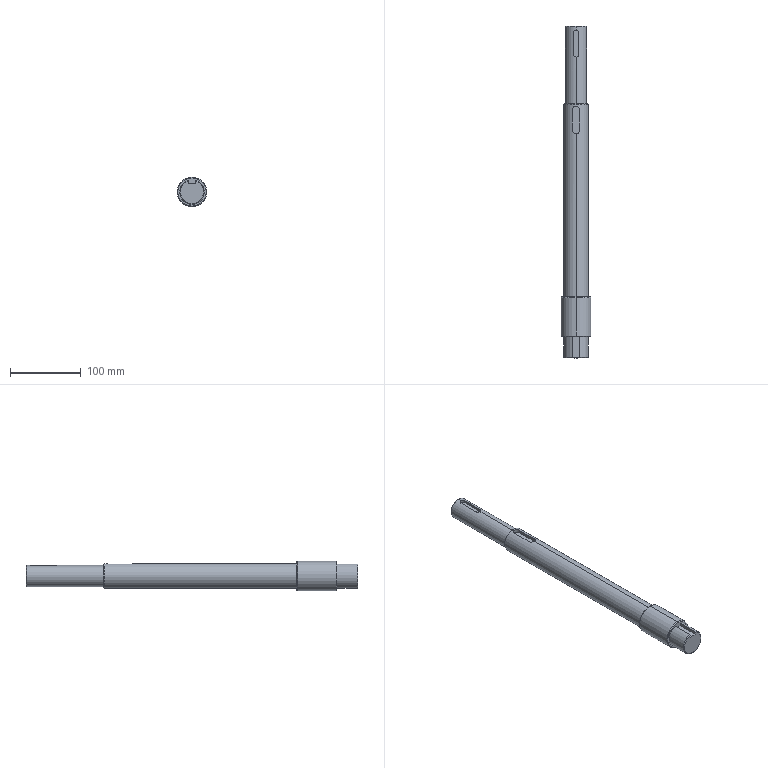Part | SolidWorks | features ICE 6, Chamfer 2, Extrusion 1 | 1 solid | 35 faces | box 42 x 470 x 42 mm | volume 443457 mm3 | plane 14 | cylinder 12 | cone 9 | commonest cylinder face diameters 35 x4 8 x2 10 x2 30 x2 42 x2
STEP:
#1=CARTESIAN_POINT('',(0.,470.,14.));
#2=VERTEX_POINT('',#1);
#3=CARTESIAN_POINT('',(0.,470.,-14.));
#4=VERTEX_POINT('',#3);
#5=CARTESIAN_POINT('',(0.,470.,0.));
#6=DIRECTION('',(0.,1.,0.));
#7=DIRECTION('',(0.,0.,1.));
#8=AXIS2_PLACEMENT_3D('',#5,#6,#7);
#9=CIRCLE('',#8,14.);
#10=EDGE_CURVE('',#2,#4,#9,.T.);
#11=ORIENTED_EDGE('',*,*,#10,.F.);
#12=CARTESIAN_POINT('',(0.,469.,15.));
#13=VERTEX_POINT('',#12);
#14=CARTESIAN_POINT('',(0.,470.,14.));
#15=DIRECTION('',(0.,-0.7071,0.7071));
#16=VECTOR('',#15,1000.);
#17=LINE('',#14,#16);
#18=EDGE_CURVE('',#2,#13,#17,.T.);
#19=ORIENTED_EDGE('',*,*,#18,.T.);
#20=CARTESIAN_POINT('',(0.,469.,-15.));
#21=VERTEX_POINT('',#20);
#22=CARTESIAN_POINT('',(0.,469.,0.));
#23=DIRECTION('',(0.,-1.,0.));
#24=DIRECTION('',(0.,0.,1.));
#25=AXIS2_PLACEMENT_3D('',#22,#23,#24);
#26=CIRCLE('',#25,15.);
#27=EDGE_CURVE('',#21,#13,#26,.T.);
#28=ORIENTED_EDGE('',*,*,#27,.F.);
#29=CARTESIAN_POINT('',(0.,470.,-14.));
#30=DIRECTION('',(0.,-0.7071,-0.7071));
#31=VECTOR('',#30,1000.);
#32=LINE('',#29,#31);
#33=EDGE_CURVE('',#4,#21,#32,.T.);
#34=ORIENTED_EDGE('',*,*,#33,.F.);
#35=EDGE_LOOP('',(#11,#19,#28,#34));
#36=FACE_OUTER_BOUND('',#35,.T.);
#37=CARTESIAN_POINT('',(0.,470.,0.));
#38=DIRECTION('',(0.,-1.,0.));
#39=DIRECTION('',(0.,0.,-1.));
#40=AXIS2_PLACEMENT_3D('',#37,#38,#39);
#41=CONICAL_SURFACE('',#40,14.,0.7854);
#42=ADVANCED_FACE('',(#36),#41,.T.);
#43=CARTESIAN_POINT('',(0.,360.,16.5));
#44=VERTEX_POINT('',#43);
#45=CARTESIAN_POINT('',(0.,360.,-16.5));
#46=VERTEX_POINT('',#45);
#47=CARTESIAN_POINT('',(0.,360.,0.));
#48=DIRECTION('',(0.,1.,0.));
#49=DIRECTION('',(0.,0.,1.));
#50=AXIS2_PLACEMENT_3D('',#47,#48,#49);
#51=CIRCLE('',#50,16.5);
#52=EDGE_CURVE('',#44,#46,#51,.T.);
#53=ORIENTED_EDGE('',*,*,#52,.F.);
#54=CARTESIAN_POINT('',(0.,359.,17.5));
#55=VERTEX_POINT('',#54);
#56=CARTESIAN_POINT('',(0.,360.,16.5));
#57=DIRECTION('',(0.,-0.7071,0.7071));
#58=VECTOR('',#57,1000.);
#59=LINE('',#56,#58);
#60=EDGE_CURVE('',#44,#55,#59,.T.);
#61=ORIENTED_EDGE('',*,*,#60,.T.);
#62=CARTESIAN_POINT('',(0.,359.,-17.5));
#63=VERTEX_POINT('',#62);
#64=CARTESIAN_POINT('',(0.,359.,0.));
#65=DIRECTION('',(0.,-1.,0.));
#66=DIRECTION('',(0.,0.,1.));
#67=AXIS2_PLACEMENT_3D('',#64,#65,#66);
#68=CIRCLE('',#67,17.5);
#69=EDGE_CURVE('',#63,#55,#68,.T.);
#70=ORIENTED_EDGE('',*,*,#69,.F.);
#71=CARTESIAN_POINT('',(0.,360.,-16.5));
#72=DIRECTION('',(0.,-0.7071,-0.7071));
#73=VECTOR('',#72,1000.);
#74=LINE('',#71,#73);
#75=EDGE_CURVE('',#46,#63,#74,.T.);
#76=ORIENTED_EDGE('',*,*,#75,.F.);
#77=EDGE_LOOP('',(#53,#61,#70,#76));
#78=FACE_OUTER_BOUND('',#77,.T.);
#79=CARTESIAN_POINT('',(0.,360.,0.));
#80=DIRECTION('',(0.,-1.,0.));
#81=DIRECTION('',(0.,0.,-1.));
#82=AXIS2_PLACEMENT_3D('',#79,#80,#81);
#83=CONICAL_SURFACE('',#82,16.5,0.7854);
#84=ADVANCED_FACE('',(#78),#83,.T.);
#85=CARTESIAN_POINT('',(0.,86.5,20.));
#86=VERTEX_POINT('',#85);
#87=CARTESIAN_POINT('',(0.,86.5,-20.));
#88=VERTEX_POINT('',#87);
#89=CARTESIAN_POINT('',(0.,86.5,0.));
#90=DIRECTION('',(0.,1.,0.));
#91=DIRECTION('',(0.,0.,1.));
#92=AXIS2_PLACEMENT_3D('',#89,#90,#91);
#93=CIRCLE('',#92,20.);
#94=EDGE_CURVE('',#86,#88,#93,.T.);
#95=ORIENTED_EDGE('',*,*,#94,.F.);
#96=CARTESIAN_POINT('',(0.,85.5,21.));
#97=VERTEX_POINT('',#96);
#98=CARTESIAN_POINT('',(0.,86.5,20.));
#99=DIRECTION('',(0.,-0.7071,0.7071));
#100=VECTOR('',#99,1000.);
#101=LINE('',#98,#100);
#102=EDGE_CURVE('',#86,#97,#101,.T.);
#103=ORIENTED_EDGE('',*,*,#102,.T.);
#104=CARTESIAN_POINT('',(0.,85.5,-21.));
#105=VERTEX_POINT('',#104);
#106=CARTESIAN_POINT('',(0.,85.5,0.));
#107=DIRECTION('',(0.,-1.,0.));
#108=DIRECTION('',(0.,0.,1.));
#109=AXIS2_PLACEMENT_3D('',#106,#107,#108);
#110=CIRCLE('',#109,21.);
#111=EDGE_CURVE('',#105,#97,#110,.T.);
#112=ORIENTED_EDGE('',*,*,#111,.F.);
#113=CARTESIAN_POINT('',(0.,86.5,-20.));
#114=DIRECTION('',(0.,-0.7071,-0.7071));
#115=VECTOR('',#114,1000.);
#116=LINE('',#113,#115);
#117=EDGE_CURVE('',#88,#105,#116,.T.);
#118=ORIENTED_EDGE('',*,*,#117,.F.);
#119=EDGE_LOOP('',(#95,#103,#112,#118));
#120=FACE_OUTER_BOUND('',#119,.T.);
#121=CARTESIAN_POINT('',(0.,86.5,0.));
#122=DIRECTION('',(0.,-1.,0.));
#123=DIRECTION('',(0.,0.,-1.));
#124=AXIS2_PLACEMENT_3D('',#121,#122,#123);
#125=CONICAL_SURFACE('',#124,20.,0.7854);
#126=ADVANCED_FACE('',(#120),#125,.T.);
#127=CARTESIAN_POINT('',(0.,30.,-20.));
#128=VERTEX_POINT('',#127);
#129=CARTESIAN_POINT('',(0.,30.,20.));
#130=VERTEX_POINT('',#129);
#131=CARTESIAN_POINT('',(0.,30.,0.));
#132=DIRECTION('',(0.,-1.,0.));
#133=DIRECTION('',(0.,0.,1.));
#134=AXIS2_PLACEMENT_3D('',#131,#132,#133);
#135=CIRCLE('',#134,20.);
#136=EDGE_CURVE('',#128,#130,#135,.T.);
#137=ORIENTED_EDGE('',*,*,#136,.F.);
#138=CARTESIAN_POINT('',(0.,31.,-21.));
#139=VERTEX_POINT('',#138);
#140=CARTESIAN_POINT('',(0.,31.,-21.));
#141=DIRECTION('',(0.,0.7071,-0.7071));
#142=VECTOR('',#141,1000.);
#143=LINE('',#140,#142);
#144=EDGE_CURVE('',#128,#139,#143,.T.);
#145=ORIENTED_EDGE('',*,*,#144,.T.);
#146=CARTESIAN_POINT('',(0.,31.,21.));
#147=VERTEX_POINT('',#146);
#148=CARTESIAN_POINT('',(0.,31.,0.));
#149=DIRECTION('',(0.,1.,0.));
#150=DIRECTION('',(0.,0.,1.));
#151=AXIS2_PLACEMENT_3D('',#148,#149,#150);
#152=CIRCLE('',#151,21.);
#153=EDGE_CURVE('',#147,#139,#152,.T.);
#154=ORIENTED_EDGE('',*,*,#153,.F.);
#155=CARTESIAN_POINT('',(0.,31.,21.));
#156=DIRECTION('',(0.,0.7071,0.7071));
#157=VECTOR('',#156,1000.);
#158=LINE('',#155,#157);
#159=EDGE_CURVE('',#130,#147,#158,.T.);
#160=ORIENTED_EDGE('',*,*,#159,.F.);
#161=EDGE_LOOP('',(#137,#145,#154,#160));
#162=FACE_OUTER_BOUND('',#161,.T.);
#163=CARTESIAN_POINT('',(0.,31.,0.));
#164=DIRECTION('',(0.,1.,0.));
#165=DIRECTION('',(0.,0.,1.));
#166=AXIS2_PLACEMENT_3D('',#163,#164,#165);
#167=CONICAL_SURFACE('',#166,21.,0.7854);
#168=ADVANCED_FACE('',(#162),#167,.T.);
#169=ORIENTED_EDGE('',*,*,#27,.T.);
#170=CARTESIAN_POINT('',(0.,464.,15.));
#171=VERTEX_POINT('',#170);
#172=CARTESIAN_POINT('',(0.,470.,15.));
#173=DIRECTION('',(0.,-1.,0.));
#174=VECTOR('',#173,1000.);
#175=LINE('',#172,#174);
#176=EDGE_CURVE('',#13,#171,#175,.T.);
#177=ORIENTED_EDGE('',*,*,#176,.T.);
#178=CARTESIAN_POINT('',(4.,460.,14.457));
#179=VERTEX_POINT('',#178);
#180=CARTESIAN_POINT('',(0.,464.,15.));
#181=CARTESIAN_POINT('',(0.262,464.,15.));
#182=CARTESIAN_POINT('',(0.5282,463.974,14.993));
#183=CARTESIAN_POINT('',(1.042,463.871,14.966));
#184=CARTESIAN_POINT('',(1.292,463.795,14.946));
#185=CARTESIAN_POINT('',(2.02,463.492,14.871));
#186=CARTESIAN_POINT('',(2.459,463.198,14.802));
#187=CARTESIAN_POINT('',(3.014,462.643,14.695));
#188=CARTESIAN_POINT('',(3.178,462.443,14.66));
#189=CARTESIAN_POINT('',(3.467,462.011,14.594));
#190=CARTESIAN_POINT('',(3.593,461.777,14.564));
#191=CARTESIAN_POINT('',(3.794,461.295,14.513));
#192=CARTESIAN_POINT('',(3.87,461.046,14.492));
#193=CARTESIAN_POINT('',(3.973,460.531,14.464));
#194=CARTESIAN_POINT('',(4.,460.265,14.457));
#195=CARTESIAN_POINT('',(4.,460.,14.457));
#196=B_SPLINE_CURVE_WITH_KNOTS('',3,(#180,#181,#182,#183,#184,#185,#186,#187,#188,#189,#190,#191,#192,#193,#194,#195),.UNSPECIFIED.,.F.,.F.,(4,2,2,2,2,2,2,4),(0.006283,0.007068,0.007852,0.009421,0.01021,0.01099,0.01177,0.01256),.UNSPECIFIED.);
#197=EDGE_CURVE('',#171,#179,#196,.T.);
#198=ORIENTED_EDGE('',*,*,#197,.T.);
#199=CARTESIAN_POINT('',(4.,430.,14.457));
#200=VERTEX_POINT('',#199);
#201=CARTESIAN_POINT('',(4.,470.,14.457));
#202=DIRECTION('',(0.,-1.,0.));
#203=VECTOR('',#202,1000.);
#204=LINE('',#201,#203);
#205=EDGE_CURVE('',#179,#200,#204,.T.);
#206=ORIENTED_EDGE('',*,*,#205,.T.);
#207=CARTESIAN_POINT('',(0.,426.,15.));
#208=VERTEX_POINT('',#207);
#209=CARTESIAN_POINT('',(4.,430.,14.457));
#210=CARTESIAN_POINT('',(4.,429.734,14.457));
#211=CARTESIAN_POINT('',(3.974,429.473,14.464));
#212=CARTESIAN_POINT('',(3.871,428.96,14.492));
#213=CARTESIAN_POINT('',(3.794,428.706,14.513));
#214=CARTESIAN_POINT('',(3.593,428.222,14.564));
#215=CARTESIAN_POINT('',(3.47,427.992,14.594));
#216=CARTESIAN_POINT('',(3.179,427.558,14.66));
#217=CARTESIAN_POINT('',(3.011,427.354,14.696));
#218=CARTESIAN_POINT('',(2.644,426.987,14.766));
#219=CARTESIAN_POINT('',(2.443,426.822,14.801));
#220=CARTESIAN_POINT('',(2.006,426.529,14.867));
#221=CARTESIAN_POINT('',(1.775,426.406,14.897));
#222=CARTESIAN_POINT('',(1.293,426.206,14.946));
#223=CARTESIAN_POINT('',(1.04,426.129,14.966));
#224=CARTESIAN_POINT('',(0.5228,426.026,14.993));
#225=CARTESIAN_POINT('',(0.2623,426.,15.));
#226=CARTESIAN_POINT('',(0.,426.,15.));
#227=B_SPLINE_CURVE_WITH_KNOTS('',3,(#209,#210,#211,#212,#213,#214,#215,#216,#217,#218,#219,#220,#221,#222,#223,#224,#225,#226),.UNSPECIFIED.,.F.,.F.,(4,2,2,2,2,2,2,2,4),(0.,0.0007854,0.001571,0.002356,0.003142,0.003927,0.004712,0.005498,0.006283),.UNSPECIFIED.);
#228=EDGE_CURVE('',#200,#208,#227,.T.);
#229=ORIENTED_EDGE('',*,*,#228,.T.);
#230=CARTESIAN_POINT('',(0.,360.,15.));
#231=VERTEX_POINT('',#230);
#232=CARTESIAN_POINT('',(0.,470.,15.));
#233=DIRECTION('',(0.,-1.,0.));
#234=VECTOR('',#233,1000.);
#235=LINE('',#232,#234);
#236=EDGE_CURVE('',#208,#231,#235,.T.);
#237=ORIENTED_EDGE('',*,*,#236,.T.);
#238=CARTESIAN_POINT('',(0.,360.,-15.));
#239=VERTEX_POINT('',#238);
#240=CARTESIAN_POINT('',(0.,360.,0.));
#241=DIRECTION('',(0.,1.,0.));
#242=DIRECTION('',(0.,0.,1.));
#243=AXIS2_PLACEMENT_3D('',#240,#241,#242);
#244=CIRCLE('',#243,15.);
#245=EDGE_CURVE('',#231,#239,#244,.T.);
#246=ORIENTED_EDGE('',*,*,#245,.T.);
#247=CARTESIAN_POINT('',(0.,470.,-15.));
#248=DIRECTION('',(0.,-1.,0.));
#249=VECTOR('',#248,1000.);
#250=LINE('',#247,#249);
#251=EDGE_CURVE('',#21,#239,#250,.T.);
#252=ORIENTED_EDGE('',*,*,#251,.F.);
#253=EDGE_LOOP('',(#169,#177,#198,#206,#229,#237,#246,#252));
#254=FACE_OUTER_BOUND('',#253,.T.);
#255=CARTESIAN_POINT('',(0.,470.,0.));
#256=DIRECTION('',(0.,-1.,0.));
#257=DIRECTION('',(0.,0.,-1.));
#258=AXIS2_PLACEMENT_3D('',#255,#256,#257);
#259=CYLINDRICAL_SURFACE('',#258,15.);
#260=ADVANCED_FACE('',(#254),#259,.T.);
#261=ORIENTED_EDGE('',*,*,#69,.T.);
#262=CARTESIAN_POINT('',(0.,356.5,17.5));
#263=VERTEX_POINT('',#262);
#264=CARTESIAN_POINT('',(0.,360.,17.5));
#265=DIRECTION('',(0.,-1.,0.));
#266=VECTOR('',#265,1000.);
#267=LINE('',#264,#266);
#268=EDGE_CURVE('',#55,#263,#267,.T.);
#269=ORIENTED_EDGE('',*,*,#268,.T.);
#270=CARTESIAN_POINT('',(5.,351.5,16.771));
#271=VERTEX_POINT('',#270);
#272=CARTESIAN_POINT('',(0.,356.5,17.5));
#273=CARTESIAN_POINT('',(0.3278,356.5,17.5));
#274=CARTESIAN_POINT('',(0.6608,356.467,17.49));
#275=CARTESIAN_POINT('',(1.303,356.338,17.454));
#276=CARTESIAN_POINT('',(1.615,356.243,17.428));
#277=CARTESIAN_POINT('',(2.222,355.991,17.361));
#278=CARTESIAN_POINT('',(2.512,355.835,17.321));
#279=CARTESIAN_POINT('',(3.051,355.474,17.234));
#280=CARTESIAN_POINT('',(3.305,355.266,17.187));
#281=CARTESIAN_POINT('',(3.767,354.804,17.091));
#282=CARTESIAN_POINT('',(3.972,354.554,17.044));
#283=CARTESIAN_POINT('',(4.334,354.014,16.956));
#284=CARTESIAN_POINT('',(4.491,353.722,16.914));
#285=CARTESIAN_POINT('',(4.742,353.12,16.846));
#286=CARTESIAN_POINT('',(4.837,352.808,16.818));
#287=CARTESIAN_POINT('',(4.967,352.164,16.781));
#288=CARTESIAN_POINT('',(5.,351.832,16.771));
#289=CARTESIAN_POINT('',(5.,351.5,16.771));
#290=B_SPLINE_CURVE_WITH_KNOTS('',3,(#272,#273,#274,#275,#276,#277,#278,#279,#280,#281,#282,#283,#284,#285,#286,#287,#288,#289),.UNSPECIFIED.,.F.,.F.,(4,2,2,2,2,2,2,2,4),(0.007859,0.008841,0.009822,0.0108,0.01178,0.01277,0.01375,0.01473,0.01571),.UNSPECIFIED.);
#291=EDGE_CURVE('',#263,#271,#290,.T.);
#292=ORIENTED_EDGE('',*,*,#291,.T.);
#293=CARTESIAN_POINT('',(5.,322.5,16.771));
#294=VERTEX_POINT('',#293);
#295=CARTESIAN_POINT('',(5.,360.,16.771));
#296=DIRECTION('',(0.,-1.,0.));
#297=VECTOR('',#296,1000.);
#298=LINE('',#295,#297);
#299=EDGE_CURVE('',#271,#294,#298,.T.);
#300=ORIENTED_EDGE('',*,*,#299,.T.);
#301=CARTESIAN_POINT('',(0.,317.5,17.5));
#302=VERTEX_POINT('',#301);
#303=CARTESIAN_POINT('',(5.,322.5,16.771));
#304=CARTESIAN_POINT('',(5.,322.168,16.771));
#305=CARTESIAN_POINT('',(4.967,321.841,16.78));
#306=CARTESIAN_POINT('',(4.839,321.2,16.818));
#307=CARTESIAN_POINT('',(4.742,320.881,16.846));
#308=CARTESIAN_POINT('',(4.49,320.276,16.915));
#309=CARTESIAN_POINT('',(4.337,319.99,16.955));
#310=CARTESIAN_POINT('',(3.974,319.448,17.044));
#311=CARTESIAN_POINT('',(3.764,319.192,17.092));
#312=CARTESIAN_POINT('',(3.305,318.734,17.187));
#313=CARTESIAN_POINT('',(3.054,318.527,17.234));
#314=CARTESIAN_POINT('',(2.507,318.162,17.322));
#315=CARTESIAN_POINT('',(2.219,318.008,17.361));
#316=CARTESIAN_POINT('',(1.768,317.82,17.411));
#317=CARTESIAN_POINT('',(1.614,317.765,17.426));
#318=CARTESIAN_POINT('',(1.3,317.669,17.452));
#319=CARTESIAN_POINT('',(1.139,317.629,17.464));
#320=CARTESIAN_POINT('',(0.6539,317.532,17.491));
#321=CARTESIAN_POINT('',(0.3282,317.5,17.5));
#322=CARTESIAN_POINT('',(0.,317.5,17.5));
#323=B_SPLINE_CURVE_WITH_KNOTS('',3,(#303,#304,#305,#306,#307,#308,#309,#310,#311,#312,#313,#314,#315,#316,#317,#318,#319,#320,#321,#322),.UNSPECIFIED.,.F.,.F.,(4,2,2,2,2,2,2,2,2,4),(0.,0.0009824,0.001965,0.002947,0.00393,0.004912,0.005894,0.006386,0.006877,0.007859),.UNSPECIFIED.);
#324=EDGE_CURVE('',#294,#302,#323,.T.);
#325=ORIENTED_EDGE('',*,*,#324,.T.);
#326=CARTESIAN_POINT('',(0.,86.5,17.5));
#327=VERTEX_POINT('',#326);
#328=CARTESIAN_POINT('',(0.,360.,17.5));
#329=DIRECTION('',(0.,-1.,0.));
#330=VECTOR('',#329,1000.);
#331=LINE('',#328,#330);
#332=EDGE_CURVE('',#302,#327,#331,.T.);
#333=ORIENTED_EDGE('',*,*,#332,.T.);
#334=CARTESIAN_POINT('',(0.,86.5,-17.5));
#335=VERTEX_POINT('',#334);
#336=CARTESIAN_POINT('',(0.,86.5,0.));
#337=DIRECTION('',(0.,1.,0.));
#338=DIRECTION('',(0.,0.,1.));
#339=AXIS2_PLACEMENT_3D('',#336,#337,#338);
#340=CIRCLE('',#339,17.5);
#341=EDGE_CURVE('',#327,#335,#340,.T.);
#342=ORIENTED_EDGE('',*,*,#341,.T.);
#343=CARTESIAN_POINT('',(0.,360.,-17.5));
#344=DIRECTION('',(0.,-1.,0.));
#345=VECTOR('',#344,1000.);
#346=LINE('',#343,#345);
#347=EDGE_CURVE('',#63,#335,#346,.T.);
#348=ORIENTED_EDGE('',*,*,#347,.F.);
#349=EDGE_LOOP('',(#261,#269,#292,#300,#325,#333,#342,#348));
#350=FACE_OUTER_BOUND('',#349,.T.);
#351=CARTESIAN_POINT('',(0.,360.,0.));
#352=DIRECTION('',(0.,-1.,0.));
#353=DIRECTION('',(0.,0.,-1.));
#354=AXIS2_PLACEMENT_3D('',#351,#352,#353);
#355=CYLINDRICAL_SURFACE('',#354,17.5);
#356=ADVANCED_FACE('',(#350),#355,.T.);
#357=ORIENTED_EDGE('',*,*,#111,.T.);
#358=CARTESIAN_POINT('',(0.,86.5,21.));
#359=DIRECTION('',(0.,-1.,0.));
#360=VECTOR('',#359,1000.);
#361=LINE('',#358,#360);
#362=EDGE_CURVE('',#97,#147,#361,.T.);
#363=ORIENTED_EDGE('',*,*,#362,.T.);
#364=ORIENTED_EDGE('',*,*,#153,.T.);
#365=CARTESIAN_POINT('',(0.,86.5,-21.));
#366=DIRECTION('',(0.,-1.,0.));
#367=VECTOR('',#366,1000.);
#368=LINE('',#365,#367);
#369=EDGE_CURVE('',#105,#139,#368,.T.);
#370=ORIENTED_EDGE('',*,*,#369,.F.);
#371=EDGE_LOOP('',(#357,#363,#364,#370));
#372=FACE_OUTER_BOUND('',#371,.T.);
#373=CARTESIAN_POINT('',(0.,86.5,0.));
#374=DIRECTION('',(0.,-1.,0.));
#375=DIRECTION('',(0.,0.,-1.));
#376=AXIS2_PLACEMENT_3D('',#373,#374,#375);
#377=CYLINDRICAL_SURFACE('',#376,21.);
#378=ADVANCED_FACE('',(#372),#377,.T.);
#379=CARTESIAN_POINT('',(0.,30.,-17.5));
#380=VERTEX_POINT('',#379);
#381=CARTESIAN_POINT('',(-5.,30.,16.771));
#382=VERTEX_POINT('',#381);
#383=CARTESIAN_POINT('',(0.,30.,0.));
#384=DIRECTION('',(0.,1.,0.));
#385=DIRECTION('',(0.,0.,1.));
#386=AXIS2_PLACEMENT_3D('',#383,#384,#385);
#387=CIRCLE('',#386,17.5);
#388=EDGE_CURVE('',#380,#382,#387,.T.);
#389=ORIENTED_EDGE('',*,*,#388,.F.);
#390=CARTESIAN_POINT('',(0.,1.,-17.5));
#391=VERTEX_POINT('',#390);
#392=CARTESIAN_POINT('',(0.,30.,-17.5));
#393=DIRECTION('',(0.,-1.,0.));
#394=VECTOR('',#393,1000.);
#395=LINE('',#392,#394);
#396=EDGE_CURVE('',#380,#391,#395,.T.);
#397=ORIENTED_EDGE('',*,*,#396,.T.);
#398=CARTESIAN_POINT('',(-5.,1.,16.771));
#399=VERTEX_POINT('',#398);
#400=CARTESIAN_POINT('',(0.,1.,0.));
#401=DIRECTION('',(0.,1.,0.));
#402=DIRECTION('',(0.,0.,1.));
#403=AXIS2_PLACEMENT_3D('',#400,#401,#402);
#404=CIRCLE('',#403,17.5);
#405=EDGE_CURVE('',#391,#399,#404,.T.);
#406=ORIENTED_EDGE('',*,*,#405,.T.);
#407=CARTESIAN_POINT('',(-5.,30.,16.771));
#408=DIRECTION('',(0.,1.,0.));
#409=VECTOR('',#408,1000.);
#410=LINE('',#407,#409);
#411=EDGE_CURVE('',#399,#382,#410,.T.);
#412=ORIENTED_EDGE('',*,*,#411,.T.);
#413=EDGE_LOOP('',(#389,#397,#406,#412));
#414=FACE_OUTER_BOUND('',#413,.T.);
#415=CARTESIAN_POINT('',(0.,30.,0.));
#416=DIRECTION('',(0.,-1.,0.));
#417=DIRECTION('',(0.,0.,-1.));
#418=AXIS2_PLACEMENT_3D('',#415,#416,#417);
#419=CYLINDRICAL_SURFACE('',#418,17.5);
#420=ADVANCED_FACE('',(#414),#419,.T.);
#421=CARTESIAN_POINT('',(0.,360.,0.));
#422=DIRECTION('',(0.,1.,0.));
#423=DIRECTION('',(0.,0.,1.));
#424=AXIS2_PLACEMENT_3D('',#421,#422,#423);
#425=CIRCLE('',#424,16.5);
#426=EDGE_CURVE('',#46,#44,#425,.T.);
#427=ORIENTED_EDGE('',*,*,#426,.T.);
#428=ORIENTED_EDGE('',*,*,#52,.T.);
#429=EDGE_LOOP('',(#427,#428));
#430=FACE_OUTER_BOUND('',#429,.T.);
#431=CARTESIAN_POINT('',(0.,360.,0.));
#432=DIRECTION('',(0.,1.,0.));
#433=DIRECTION('',(0.,0.,1.));
#434=AXIS2_PLACEMENT_3D('',#431,#432,#433);
#435=CIRCLE('',#434,15.);
#436=EDGE_CURVE('',#239,#231,#435,.T.);
#437=ORIENTED_EDGE('',*,*,#436,.F.);
#438=ORIENTED_EDGE('',*,*,#245,.F.);
#439=EDGE_LOOP('',(#437,#438));
#440=FACE_BOUND('',#439,.T.);
#441=CARTESIAN_POINT('',(0.,360.,0.));
#442=DIRECTION('',(0.,1.,0.));
#443=DIRECTION('',(0.,0.,1.));
#444=AXIS2_PLACEMENT_3D('',#441,#442,#443);
#445=PLANE('',#444);
#446=ADVANCED_FACE('',(#430,#440),#445,.T.);
#447=CARTESIAN_POINT('',(0.,86.5,0.));
#448=DIRECTION('',(0.,1.,0.));
#449=DIRECTION('',(0.,0.,1.));
#450=AXIS2_PLACEMENT_3D('',#447,#448,#449);
#451=CIRCLE('',#450,20.);
#452=EDGE_CURVE('',#88,#86,#451,.T.);
#453=ORIENTED_EDGE('',*,*,#452,.T.);
#454=ORIENTED_EDGE('',*,*,#94,.T.);
#455=EDGE_LOOP('',(#453,#454));
#456=FACE_OUTER_BOUND('',#455,.T.);
#457=CARTESIAN_POINT('',(0.,86.5,0.));
#458=DIRECTION('',(0.,1.,0.));
#459=DIRECTION('',(0.,0.,1.));
#460=AXIS2_PLACEMENT_3D('',#457,#458,#459);
#461=CIRCLE('',#460,17.5);
#462=EDGE_CURVE('',#335,#327,#461,.T.);
#463=ORIENTED_EDGE('',*,*,#462,.F.);
#464=ORIENTED_EDGE('',*,*,#341,.F.);
#465=EDGE_LOOP('',(#463,#464));
#466=FACE_BOUND('',#465,.T.);
#467=CARTESIAN_POINT('',(0.,86.5,0.));
#468=DIRECTION('',(0.,1.,0.));
#469=DIRECTION('',(0.,0.,1.));
#470=AXIS2_PLACEMENT_3D('',#467,#468,#469);
#471=PLANE('',#470);
#472=ADVANCED_FACE('',(#456,#466),#471,.T.);
#473=ORIENTED_EDGE('',*,*,#396,.F.);
#474=CARTESIAN_POINT('',(5.,30.,16.771));
#475=VERTEX_POINT('',#474);
#476=CARTESIAN_POINT('',(0.,30.,0.));
#477=DIRECTION('',(0.,1.,0.));
#478=DIRECTION('',(0.,0.,1.));
#479=AXIS2_PLACEMENT_3D('',#476,#477,#478);
#480=CIRCLE('',#479,17.5);
#481=EDGE_CURVE('',#475,#380,#480,.T.);
#482=ORIENTED_EDGE('',*,*,#481,.F.);
#483=CARTESIAN_POINT('',(5.,1.,16.771));
#484=VERTEX_POINT('',#483);
#485=CARTESIAN_POINT('',(5.,30.,16.771));
#486=DIRECTION('',(0.,-1.,0.));
#487=VECTOR('',#486,1000.);
#488=LINE('',#485,#487);
#489=EDGE_CURVE('',#475,#484,#488,.T.);
#490=ORIENTED_EDGE('',*,*,#489,.T.);
#491=CARTESIAN_POINT('',(0.,1.,0.));
#492=DIRECTION('',(0.,1.,0.));
#493=DIRECTION('',(0.,0.,1.));
#494=AXIS2_PLACEMENT_3D('',#491,#492,#493);
#495=CIRCLE('',#494,17.5);
#496=EDGE_CURVE('',#484,#391,#495,.T.);
#497=ORIENTED_EDGE('',*,*,#496,.T.);
#498=EDGE_LOOP('',(#473,#482,#490,#497));
#499=FACE_OUTER_BOUND('',#498,.T.);
#500=CARTESIAN_POINT('',(0.,30.,0.));
#501=DIRECTION('',(0.,-1.,0.));
#502=DIRECTION('',(0.,0.,-1.));
#503=AXIS2_PLACEMENT_3D('',#500,#501,#502);
#504=CYLINDRICAL_SURFACE('',#503,17.5);
#505=ADVANCED_FACE('',(#499),#504,.T.);
#506=CARTESIAN_POINT('',(-5.,0.,12.5));
#507=VERTEX_POINT('',#506);
#508=CARTESIAN_POINT('',(5.,0.,12.5));
#509=VERTEX_POINT('',#508);
#510=CARTESIAN_POINT('',(-5.,0.,12.5));
#511=DIRECTION('',(1.,0.,0.));
#512=VECTOR('',#511,1000.);
#513=LINE('',#510,#512);
#514=EDGE_CURVE('',#507,#509,#513,.T.);
#515=ORIENTED_EDGE('',*,*,#514,.F.);
#516=CARTESIAN_POINT('',(-5.,0.,15.724));
#517=VERTEX_POINT('',#516);
#518=CARTESIAN_POINT('',(-5.,0.,22.5));
#519=DIRECTION('',(0.,0.,-1.));
#520=VECTOR('',#519,1000.);
#521=LINE('',#518,#520);
#522=EDGE_CURVE('',#517,#507,#521,.T.);
#523=ORIENTED_EDGE('',*,*,#522,.F.);
#524=CARTESIAN_POINT('',(5.,0.,15.724));
#525=VERTEX_POINT('',#524);
#526=CARTESIAN_POINT('',(0.,0.,0.));
#527=DIRECTION('',(0.,-1.,0.));
#528=DIRECTION('',(0.,0.,1.));
#529=AXIS2_PLACEMENT_3D('',#526,#527,#528);
#530=CIRCLE('',#529,16.5);
#531=EDGE_CURVE('',#517,#525,#530,.T.);
#532=ORIENTED_EDGE('',*,*,#531,.T.);
#533=CARTESIAN_POINT('',(5.,0.,22.5));
#534=DIRECTION('',(0.,0.,1.));
#535=VECTOR('',#534,1000.);
#536=LINE('',#533,#535);
#537=EDGE_CURVE('',#509,#525,#536,.T.);
#538=ORIENTED_EDGE('',*,*,#537,.F.);
#539=EDGE_LOOP('',(#515,#523,#532,#538));
#540=FACE_OUTER_BOUND('',#539,.T.);
#541=CARTESIAN_POINT('',(0.,0.,0.));
#542=DIRECTION('',(0.,1.,0.));
#543=DIRECTION('',(0.,0.,1.));
#544=AXIS2_PLACEMENT_3D('',#541,#542,#543);
#545=PLANE('',#544);
#546=ADVANCED_FACE('',(#540),#545,.F.);
#547=CARTESIAN_POINT('',(0.,30.,0.));
#548=DIRECTION('',(0.,-1.,0.));
#549=DIRECTION('',(0.,0.,1.));
#550=AXIS2_PLACEMENT_3D('',#547,#548,#549);
#551=CIRCLE('',#550,20.);
#552=EDGE_CURVE('',#130,#128,#551,.T.);
#553=ORIENTED_EDGE('',*,*,#552,.T.);
#554=ORIENTED_EDGE('',*,*,#136,.T.);
#555=EDGE_LOOP('',(#553,#554));
#556=FACE_OUTER_BOUND('',#555,.T.);
#557=ORIENTED_EDGE('',*,*,#481,.T.);
#558=ORIENTED_EDGE('',*,*,#388,.T.);
#559=CARTESIAN_POINT('',(-5.,30.,12.5));
#560=VERTEX_POINT('',#559);
#561=CARTESIAN_POINT('',(-5.,30.,22.5));
#562=DIRECTION('',(0.,0.,-1.));
#563=VECTOR('',#562,1000.);
#564=LINE('',#561,#563);
#565=EDGE_CURVE('',#382,#560,#564,.T.);
#566=ORIENTED_EDGE('',*,*,#565,.T.);
#567=CARTESIAN_POINT('',(5.,30.,12.5));
#568=VERTEX_POINT('',#567);
#569=CARTESIAN_POINT('',(-5.,30.,12.5));
#570=DIRECTION('',(1.,0.,0.));
#571=VECTOR('',#570,1000.);
#572=LINE('',#569,#571);
#573=EDGE_CURVE('',#560,#568,#572,.T.);
#574=ORIENTED_EDGE('',*,*,#573,.T.);
#575=CARTESIAN_POINT('',(5.,30.,22.5));
#576=DIRECTION('',(0.,0.,1.));
#577=VECTOR('',#576,1000.);
#578=LINE('',#575,#577);
#579=EDGE_CURVE('',#568,#475,#578,.T.);
#580=ORIENTED_EDGE('',*,*,#579,.T.);
#581=EDGE_LOOP('',(#557,#558,#566,#574,#580));
#582=FACE_BOUND('',#581,.T.);
#583=CARTESIAN_POINT('',(0.,30.,0.));
#584=DIRECTION('',(0.,1.,0.));
#585=DIRECTION('',(0.,0.,1.));
#586=AXIS2_PLACEMENT_3D('',#583,#584,#585);
#587=PLANE('',#586);
#588=ADVANCED_FACE('',(#556,#582),#587,.F.);
#589=ORIENTED_EDGE('',*,*,#362,.F.);
#590=CARTESIAN_POINT('',(0.,85.5,0.));
#591=DIRECTION('',(0.,-1.,0.));
#592=DIRECTION('',(0.,0.,1.));
#593=AXIS2_PLACEMENT_3D('',#590,#591,#592);
#594=CIRCLE('',#593,21.);
#595=EDGE_CURVE('',#97,#105,#594,.T.);
#596=ORIENTED_EDGE('',*,*,#595,.T.);
#597=ORIENTED_EDGE('',*,*,#369,.T.);
#598=CARTESIAN_POINT('',(0.,31.,0.));
#599=DIRECTION('',(0.,1.,0.));
#600=DIRECTION('',(0.,0.,1.));
#601=AXIS2_PLACEMENT_3D('',#598,#599,#600);
#602=CIRCLE('',#601,21.);
#603=EDGE_CURVE('',#139,#147,#602,.T.);
#604=ORIENTED_EDGE('',*,*,#603,.T.);
#605=EDGE_LOOP('',(#589,#596,#597,#604));
#606=FACE_OUTER_BOUND('',#605,.T.);
#607=CARTESIAN_POINT('',(0.,86.5,0.));
#608=DIRECTION('',(0.,-1.,0.));
#609=DIRECTION('',(0.,0.,-1.));
#610=AXIS2_PLACEMENT_3D('',#607,#608,#609);
#611=CYLINDRICAL_SURFACE('',#610,21.);
#612=ADVANCED_FACE('',(#606),#611,.T.);
#613=ORIENTED_EDGE('',*,*,#268,.F.);
#614=CARTESIAN_POINT('',(0.,359.,0.));
#615=DIRECTION('',(0.,-1.,0.));
#616=DIRECTION('',(0.,0.,1.));
#617=AXIS2_PLACEMENT_3D('',#614,#615,#616);
#618=CIRCLE('',#617,17.5);
#619=EDGE_CURVE('',#55,#63,#618,.T.);
#620=ORIENTED_EDGE('',*,*,#619,.T.);
#621=ORIENTED_EDGE('',*,*,#347,.T.);
#622=ORIENTED_EDGE('',*,*,#462,.T.);
#623=ORIENTED_EDGE('',*,*,#332,.F.);
#624=CARTESIAN_POINT('',(-5.,322.5,16.771));
#625=VERTEX_POINT('',#624);
#626=CARTESIAN_POINT('',(0.,317.5,17.5));
#627=CARTESIAN_POINT('',(-0.3278,317.5,17.5));
#628=CARTESIAN_POINT('',(-0.6608,317.533,17.49));
#629=CARTESIAN_POINT('',(-1.303,317.662,17.454));
#630=CARTESIAN_POINT('',(-1.615,317.757,17.428));
#631=CARTESIAN_POINT('',(-2.222,318.009,17.361));
#632=CARTESIAN_POINT('',(-2.512,318.165,17.321));
#633=CARTESIAN_POINT('',(-3.051,318.526,17.234));
#634=CARTESIAN_POINT('',(-3.305,318.734,17.187));
#635=CARTESIAN_POINT('',(-3.767,319.196,17.091));
#636=CARTESIAN_POINT('',(-3.972,319.446,17.044));
#637=CARTESIAN_POINT('',(-4.334,319.986,16.956));
#638=CARTESIAN_POINT('',(-4.491,320.278,16.914));
#639=CARTESIAN_POINT('',(-4.742,320.88,16.846));
#640=CARTESIAN_POINT('',(-4.837,321.192,16.818));
#641=CARTESIAN_POINT('',(-4.967,321.836,16.781));
#642=CARTESIAN_POINT('',(-5.,322.168,16.771));
#643=CARTESIAN_POINT('',(-5.,322.5,16.771));
#644=B_SPLINE_CURVE_WITH_KNOTS('',3,(#626,#627,#628,#629,#630,#631,#632,#633,#634,#635,#636,#637,#638,#639,#640,#641,#642,#643),.UNSPECIFIED.,.F.,.F.,(4,2,2,2,2,2,2,2,4),(0.007859,0.008841,0.009822,0.0108,0.01178,0.01277,0.01375,0.01473,0.01571),.UNSPECIFIED.);
#645=EDGE_CURVE('',#302,#625,#644,.T.);
#646=ORIENTED_EDGE('',*,*,#645,.T.);
#647=CARTESIAN_POINT('',(-5.,351.5,16.771));
#648=VERTEX_POINT('',#647);
#649=CARTESIAN_POINT('',(-5.,360.,16.771));
#650=DIRECTION('',(0.,1.,0.));
#651=VECTOR('',#650,1000.);
#652=LINE('',#649,#651);
#653=EDGE_CURVE('',#625,#648,#652,.T.);
#654=ORIENTED_EDGE('',*,*,#653,.T.);
#655=CARTESIAN_POINT('',(-5.,351.5,16.771));
#656=CARTESIAN_POINT('',(-5.,351.832,16.771));
#657=CARTESIAN_POINT('',(-4.967,352.159,16.78));
#658=CARTESIAN_POINT('',(-4.839,352.8,16.818));
#659=CARTESIAN_POINT('',(-4.742,353.119,16.846));
#660=CARTESIAN_POINT('',(-4.49,353.724,16.915));
#661=CARTESIAN_POINT('',(-4.337,354.01,16.955));
#662=CARTESIAN_POINT('',(-3.974,354.552,17.044));
#663=CARTESIAN_POINT('',(-3.764,354.808,17.092));
#664=CARTESIAN_POINT('',(-3.305,355.266,17.187));
#665=CARTESIAN_POINT('',(-3.054,355.473,17.234));
#666=CARTESIAN_POINT('',(-2.507,355.838,17.322));
#667=CARTESIAN_POINT('',(-2.219,355.992,17.361));
#668=CARTESIAN_POINT('',(-1.768,356.18,17.411));
#669=CARTESIAN_POINT('',(-1.614,356.235,17.426));
#670=CARTESIAN_POINT('',(-1.3,356.331,17.452));
#671=CARTESIAN_POINT('',(-1.139,356.371,17.464));
#672=CARTESIAN_POINT('',(-0.6539,356.468,17.491));
#673=CARTESIAN_POINT('',(-0.3282,356.5,17.5));
#674=CARTESIAN_POINT('',(0.,356.5,17.5));
#675=B_SPLINE_CURVE_WITH_KNOTS('',3,(#655,#656,#657,#658,#659,#660,#661,#662,#663,#664,#665,#666,#667,#668,#669,#670,#671,#672,#673,#674),.UNSPECIFIED.,.F.,.F.,(4,2,2,2,2,2,2,2,2,4),(0.,0.0009824,0.001965,0.002947,0.00393,0.004912,0.005894,0.006386,0.006877,0.007859),.UNSPECIFIED.);
#676=EDGE_CURVE('',#648,#263,#675,.T.);
#677=ORIENTED_EDGE('',*,*,#676,.T.);
#678=EDGE_LOOP('',(#613,#620,#621,#622,#623,#646,#654,#677));
#679=FACE_OUTER_BOUND('',#678,.T.);
#680=CARTESIAN_POINT('',(0.,360.,0.));
#681=DIRECTION('',(0.,-1.,0.));
#682=DIRECTION('',(0.,0.,-1.));
#683=AXIS2_PLACEMENT_3D('',#680,#681,#682);
#684=CYLINDRICAL_SURFACE('',#683,17.5);
#685=ADVANCED_FACE('',(#679),#684,.T.);
#686=ORIENTED_EDGE('',*,*,#176,.F.);
#687=CARTESIAN_POINT('',(0.,469.,0.));
#688=DIRECTION('',(0.,-1.,0.));
#689=DIRECTION('',(0.,0.,1.));
#690=AXIS2_PLACEMENT_3D('',#687,#688,#689);
#691=CIRCLE('',#690,15.);
#692=EDGE_CURVE('',#13,#21,#691,.T.);
#693=ORIENTED_EDGE('',*,*,#692,.T.);
#694=ORIENTED_EDGE('',*,*,#251,.T.);
#695=ORIENTED_EDGE('',*,*,#436,.T.);
#696=ORIENTED_EDGE('',*,*,#236,.F.);
#697=CARTESIAN_POINT('',(-4.,430.,14.457));
#698=VERTEX_POINT('',#697);
#699=CARTESIAN_POINT('',(0.,426.,15.));
#700=CARTESIAN_POINT('',(-0.262,426.,15.));
#701=CARTESIAN_POINT('',(-0.5282,426.026,14.993));
#702=CARTESIAN_POINT('',(-1.042,426.129,14.966));
#703=CARTESIAN_POINT('',(-1.292,426.205,14.946));
#704=CARTESIAN_POINT('',(-2.02,426.508,14.871));
#705=CARTESIAN_POINT('',(-2.459,426.802,14.802));
#706=CARTESIAN_POINT('',(-3.014,427.357,14.695));
#707=CARTESIAN_POINT('',(-3.178,427.557,14.66));
#708=CARTESIAN_POINT('',(-3.467,427.989,14.594));
#709=CARTESIAN_POINT('',(-3.593,428.223,14.564));
#710=CARTESIAN_POINT('',(-3.794,428.705,14.513));
#711=CARTESIAN_POINT('',(-3.87,428.954,14.492));
#712=CARTESIAN_POINT('',(-3.973,429.469,14.464));
#713=CARTESIAN_POINT('',(-4.,429.735,14.457));
#714=CARTESIAN_POINT('',(-4.,430.,14.457));
#715=B_SPLINE_CURVE_WITH_KNOTS('',3,(#699,#700,#701,#702,#703,#704,#705,#706,#707,#708,#709,#710,#711,#712,#713,#714),.UNSPECIFIED.,.F.,.F.,(4,2,2,2,2,2,2,4),(0.006283,0.007068,0.007852,0.009421,0.01021,0.01099,0.01177,0.01256),.UNSPECIFIED.);
#716=EDGE_CURVE('',#208,#698,#715,.T.);
#717=ORIENTED_EDGE('',*,*,#716,.T.);
#718=CARTESIAN_POINT('',(-4.,460.,14.457));
#719=VERTEX_POINT('',#718);
#720=CARTESIAN_POINT('',(-4.,470.,14.457));
#721=DIRECTION('',(0.,1.,0.));
#722=VECTOR('',#721,1000.);
#723=LINE('',#720,#722);
#724=EDGE_CURVE('',#698,#719,#723,.T.);
#725=ORIENTED_EDGE('',*,*,#724,.T.);
#726=CARTESIAN_POINT('',(-4.,460.,14.457));
#727=CARTESIAN_POINT('',(-4.,460.266,14.457));
#728=CARTESIAN_POINT('',(-3.974,460.527,14.464));
#729=CARTESIAN_POINT('',(-3.871,461.04,14.492));
#730=CARTESIAN_POINT('',(-3.794,461.294,14.513));
#731=CARTESIAN_POINT('',(-3.593,461.778,14.564));
#732=CARTESIAN_POINT('',(-3.47,462.008,14.594));
#733=CARTESIAN_POINT('',(-3.179,462.442,14.66));
#734=CARTESIAN_POINT('',(-3.011,462.646,14.696));
#735=CARTESIAN_POINT('',(-2.644,463.013,14.766));
#736=CARTESIAN_POINT('',(-2.443,463.178,14.801));
#737=CARTESIAN_POINT('',(-2.006,463.471,14.867));
#738=CARTESIAN_POINT('',(-1.775,463.594,14.897));
#739=CARTESIAN_POINT('',(-1.293,463.794,14.946));
#740=CARTESIAN_POINT('',(-1.04,463.871,14.966));
#741=CARTESIAN_POINT('',(-0.5228,463.974,14.993));
#742=CARTESIAN_POINT('',(-0.2623,464.,15.));
#743=CARTESIAN_POINT('',(0.,464.,15.));
#744=B_SPLINE_CURVE_WITH_KNOTS('',3,(#726,#727,#728,#729,#730,#731,#732,#733,#734,#735,#736,#737,#738,#739,#740,#741,#742,#743),.UNSPECIFIED.,.F.,.F.,(4,2,2,2,2,2,2,2,4),(0.,0.0007854,0.001571,0.002356,0.003142,0.003927,0.004712,0.005498,0.006283),.UNSPECIFIED.);
#745=EDGE_CURVE('',#719,#171,#744,.T.);
#746=ORIENTED_EDGE('',*,*,#745,.T.);
#747=EDGE_LOOP('',(#686,#693,#694,#695,#696,#717,#725,#746));
#748=FACE_OUTER_BOUND('',#747,.T.);
#749=CARTESIAN_POINT('',(0.,470.,0.));
#750=DIRECTION('',(0.,-1.,0.));
#751=DIRECTION('',(0.,0.,-1.));
#752=AXIS2_PLACEMENT_3D('',#749,#750,#751);
#753=CYLINDRICAL_SURFACE('',#752,15.);
#754=ADVANCED_FACE('',(#748),#753,.T.);
#755=CARTESIAN_POINT('',(0.,470.,0.));
#756=DIRECTION('',(0.,1.,0.));
#757=DIRECTION('',(0.,0.,1.));
#758=AXIS2_PLACEMENT_3D('',#755,#756,#757);
#759=CIRCLE('',#758,14.);
#760=EDGE_CURVE('',#4,#2,#759,.T.);
#761=ORIENTED_EDGE('',*,*,#760,.T.);
#762=ORIENTED_EDGE('',*,*,#10,.T.);
#763=EDGE_LOOP('',(#761,#762));
#764=FACE_OUTER_BOUND('',#763,.T.);
#765=CARTESIAN_POINT('',(0.,470.,0.));
#766=DIRECTION('',(0.,1.,0.));
#767=DIRECTION('',(0.,0.,1.));
#768=AXIS2_PLACEMENT_3D('',#765,#766,#767);
#769=PLANE('',#768);
#770=ADVANCED_FACE('',(#764),#769,.T.);
#771=CARTESIAN_POINT('',(-5.,1.,16.771));
#772=CARTESIAN_POINT('',(-5.,0.6662,16.422));
#773=CARTESIAN_POINT('',(-5.,0.3328,16.073));
#774=CARTESIAN_POINT('',(-5.,0.,15.724));
#775=B_SPLINE_CURVE_WITH_KNOTS('',3,(#771,#772,#773,#774),.UNSPECIFIED.,.F.,.F.,(4,4),(0.008313,0.00976),.UNSPECIFIED.);
#776=EDGE_CURVE('',#399,#517,#775,.T.);
#777=ORIENTED_EDGE('',*,*,#776,.F.);
#778=ORIENTED_EDGE('',*,*,#405,.F.);
#779=ORIENTED_EDGE('',*,*,#496,.F.);
#780=CARTESIAN_POINT('',(5.,0.,15.724));
#781=CARTESIAN_POINT('',(5.,0.3328,16.073));
#782=CARTESIAN_POINT('',(5.,0.6662,16.422));
#783=CARTESIAN_POINT('',(5.,1.,16.771));
#784=B_SPLINE_CURVE_WITH_KNOTS('',3,(#780,#781,#782,#783),.UNSPECIFIED.,.F.,.F.,(4,4),(0.009215,0.01066),.UNSPECIFIED.);
#785=EDGE_CURVE('',#525,#484,#784,.T.);
#786=ORIENTED_EDGE('',*,*,#785,.F.);
#787=ORIENTED_EDGE('',*,*,#531,.F.);
#788=EDGE_LOOP('',(#777,#778,#779,#786,#787));
#789=FACE_OUTER_BOUND('',#788,.T.);
#790=CARTESIAN_POINT('',(0.,1.,0.));
#791=DIRECTION('',(0.,1.,0.));
#792=DIRECTION('',(0.,0.,1.));
#793=AXIS2_PLACEMENT_3D('',#790,#791,#792);
#794=CONICAL_SURFACE('',#793,17.5,0.7854);
#795=ADVANCED_FACE('',(#789),#794,.T.);
#796=ORIENTED_EDGE('',*,*,#144,.F.);
#797=ORIENTED_EDGE('',*,*,#552,.F.);
#798=ORIENTED_EDGE('',*,*,#159,.T.);
#799=ORIENTED_EDGE('',*,*,#603,.F.);
#800=EDGE_LOOP('',(#796,#797,#798,#799));
#801=FACE_OUTER_BOUND('',#800,.T.);
#802=CARTESIAN_POINT('',(0.,31.,0.));
#803=DIRECTION('',(0.,1.,0.));
#804=DIRECTION('',(0.,0.,1.));
#805=AXIS2_PLACEMENT_3D('',#802,#803,#804);
#806=CONICAL_SURFACE('',#805,21.,0.7854);
#807=ADVANCED_FACE('',(#801),#806,.T.);
#808=ORIENTED_EDGE('',*,*,#102,.F.);
#809=ORIENTED_EDGE('',*,*,#452,.F.);
#810=ORIENTED_EDGE('',*,*,#117,.T.);
#811=ORIENTED_EDGE('',*,*,#595,.F.);
#812=EDGE_LOOP('',(#808,#809,#810,#811));
#813=FACE_OUTER_BOUND('',#812,.T.);
#814=CARTESIAN_POINT('',(0.,86.5,0.));
#815=DIRECTION('',(0.,-1.,0.));
#816=DIRECTION('',(0.,0.,-1.));
#817=AXIS2_PLACEMENT_3D('',#814,#815,#816);
#818=CONICAL_SURFACE('',#817,20.,0.7854);
#819=ADVANCED_FACE('',(#813),#818,.T.);
#820=ORIENTED_EDGE('',*,*,#60,.F.);
#821=ORIENTED_EDGE('',*,*,#426,.F.);
#822=ORIENTED_EDGE('',*,*,#75,.T.);
#823=ORIENTED_EDGE('',*,*,#619,.F.);
#824=EDGE_LOOP('',(#820,#821,#822,#823));
#825=FACE_OUTER_BOUND('',#824,.T.);
#826=CARTESIAN_POINT('',(0.,360.,0.));
#827=DIRECTION('',(0.,-1.,0.));
#828=DIRECTION('',(0.,0.,-1.));
#829=AXIS2_PLACEMENT_3D('',#826,#827,#828);
#830=CONICAL_SURFACE('',#829,16.5,0.7854);
#831=ADVANCED_FACE('',(#825),#830,.T.);
#832=ORIENTED_EDGE('',*,*,#18,.F.);
#833=ORIENTED_EDGE('',*,*,#760,.F.);
#834=ORIENTED_EDGE('',*,*,#33,.T.);
#835=ORIENTED_EDGE('',*,*,#692,.F.);
#836=EDGE_LOOP('',(#832,#833,#834,#835));
#837=FACE_OUTER_BOUND('',#836,.T.);
#838=CARTESIAN_POINT('',(0.,470.,0.));
#839=DIRECTION('',(0.,-1.,0.));
#840=DIRECTION('',(0.,0.,-1.));
#841=AXIS2_PLACEMENT_3D('',#838,#839,#840);
#842=CONICAL_SURFACE('',#841,14.,0.7854);
#843=ADVANCED_FACE('',(#837),#842,.T.);
#844=ORIENTED_EDGE('',*,*,#776,.T.);
#845=ORIENTED_EDGE('',*,*,#522,.T.);
#846=CARTESIAN_POINT('',(-5.,30.,12.5));
#847=DIRECTION('',(0.,-1.,0.));
#848=VECTOR('',#847,1000.);
#849=LINE('',#846,#848);
#850=EDGE_CURVE('',#560,#507,#849,.T.);
#851=ORIENTED_EDGE('',*,*,#850,.F.);
#852=ORIENTED_EDGE('',*,*,#565,.F.);
#853=ORIENTED_EDGE('',*,*,#411,.F.);
#854=EDGE_LOOP('',(#844,#845,#851,#852,#853));
#855=FACE_OUTER_BOUND('',#854,.T.);
#856=CARTESIAN_POINT('',(-5.,30.,22.5));
#857=DIRECTION('',(-1.,0.,0.));
#858=DIRECTION('',(0.,0.,1.));
#859=AXIS2_PLACEMENT_3D('',#856,#857,#858);
#860=PLANE('',#859);
#861=ADVANCED_FACE('',(#855),#860,.F.);
#862=ORIENTED_EDGE('',*,*,#579,.F.);
#863=CARTESIAN_POINT('',(5.,30.,12.5));
#864=DIRECTION('',(0.,-1.,0.));
#865=VECTOR('',#864,1000.);
#866=LINE('',#863,#865);
#867=EDGE_CURVE('',#568,#509,#866,.T.);
#868=ORIENTED_EDGE('',*,*,#867,.T.);
#869=ORIENTED_EDGE('',*,*,#537,.T.);
#870=ORIENTED_EDGE('',*,*,#785,.T.);
#871=ORIENTED_EDGE('',*,*,#489,.F.);
#872=EDGE_LOOP('',(#862,#868,#869,#870,#871));
#873=FACE_OUTER_BOUND('',#872,.T.);
#874=CARTESIAN_POINT('',(5.,30.,22.5));
#875=DIRECTION('',(1.,0.,0.));
#876=DIRECTION('',(0.,0.,-1.));
#877=AXIS2_PLACEMENT_3D('',#874,#875,#876);
#878=PLANE('',#877);
#879=ADVANCED_FACE('',(#873),#878,.F.);
#880=ORIENTED_EDGE('',*,*,#514,.T.);
#881=ORIENTED_EDGE('',*,*,#867,.F.);
#882=ORIENTED_EDGE('',*,*,#573,.F.);
#883=ORIENTED_EDGE('',*,*,#850,.T.);
#884=EDGE_LOOP('',(#880,#881,#882,#883));
#885=FACE_OUTER_BOUND('',#884,.T.);
#886=CARTESIAN_POINT('',(-5.,30.,12.5));
#887=DIRECTION('',(0.,0.,-1.));
#888=DIRECTION('',(-1.,0.,0.));
#889=AXIS2_PLACEMENT_3D('',#886,#887,#888);
#890=PLANE('',#889);
#891=ADVANCED_FACE('',(#885),#890,.F.);
#892=CARTESIAN_POINT('',(-5.,351.5,12.5));
#893=VERTEX_POINT('',#892);
#894=CARTESIAN_POINT('',(-5.,351.5,12.5));
#895=DIRECTION('',(0.,0.,1.));
#896=VECTOR('',#895,1000.);
#897=LINE('',#894,#896);
#898=EDGE_CURVE('',#893,#648,#897,.T.);
#899=ORIENTED_EDGE('',*,*,#898,.F.);
#900=CARTESIAN_POINT('',(5.,351.5,12.5));
#901=VERTEX_POINT('',#900);
#902=CARTESIAN_POINT('',(0.,351.5,12.5));
#903=DIRECTION('',(0.,0.,1.));
#904=DIRECTION('',(1.,0.,0.));
#905=AXIS2_PLACEMENT_3D('',#902,#903,#904);
#906=CIRCLE('',#905,5.);
#907=EDGE_CURVE('',#901,#893,#906,.T.);
#908=ORIENTED_EDGE('',*,*,#907,.F.);
#909=CARTESIAN_POINT('',(5.,351.5,12.5));
#910=DIRECTION('',(0.,0.,1.));
#911=VECTOR('',#910,1000.);
#912=LINE('',#909,#911);
#913=EDGE_CURVE('',#901,#271,#912,.T.);
#914=ORIENTED_EDGE('',*,*,#913,.T.);
#915=ORIENTED_EDGE('',*,*,#291,.F.);
#916=ORIENTED_EDGE('',*,*,#676,.F.);
#917=EDGE_LOOP('',(#899,#908,#914,#915,#916));
#918=FACE_OUTER_BOUND('',#917,.T.);
#919=CARTESIAN_POINT('',(0.,351.5,12.5));
#920=DIRECTION('',(0.,0.,1.));
#921=DIRECTION('',(1.,0.,0.));
#922=AXIS2_PLACEMENT_3D('',#919,#920,#921);
#923=CYLINDRICAL_SURFACE('',#922,5.);
#924=ADVANCED_FACE('',(#918),#923,.F.);
#925=ORIENTED_EDGE('',*,*,#913,.F.);
#926=CARTESIAN_POINT('',(5.,322.5,12.5));
#927=VERTEX_POINT('',#926);
#928=CARTESIAN_POINT('',(5.,351.5,12.5));
#929=DIRECTION('',(0.,1.,0.));
#930=VECTOR('',#929,1000.);
#931=LINE('',#928,#930);
#932=EDGE_CURVE('',#927,#901,#931,.T.);
#933=ORIENTED_EDGE('',*,*,#932,.F.);
#934=CARTESIAN_POINT('',(5.,322.5,12.5));
#935=DIRECTION('',(0.,0.,1.));
#936=VECTOR('',#935,1000.);
#937=LINE('',#934,#936);
#938=EDGE_CURVE('',#927,#294,#937,.T.);
#939=ORIENTED_EDGE('',*,*,#938,.T.);
#940=ORIENTED_EDGE('',*,*,#299,.F.);
#941=EDGE_LOOP('',(#925,#933,#939,#940));
#942=FACE_OUTER_BOUND('',#941,.T.);
#943=CARTESIAN_POINT('',(5.,351.5,12.5));
#944=DIRECTION('',(1.,0.,0.));
#945=DIRECTION('',(0.,1.,0.));
#946=AXIS2_PLACEMENT_3D('',#943,#944,#945);
#947=PLANE('',#946);
#948=ADVANCED_FACE('',(#942),#947,.F.);
#949=ORIENTED_EDGE('',*,*,#938,.F.);
#950=CARTESIAN_POINT('',(-5.,322.5,12.5));
#951=VERTEX_POINT('',#950);
#952=CARTESIAN_POINT('',(0.,322.5,12.5));
#953=DIRECTION('',(0.,0.,1.));
#954=DIRECTION('',(1.,0.,0.));
#955=AXIS2_PLACEMENT_3D('',#952,#953,#954);
#956=CIRCLE('',#955,5.);
#957=EDGE_CURVE('',#951,#927,#956,.T.);
#958=ORIENTED_EDGE('',*,*,#957,.F.);
#959=CARTESIAN_POINT('',(-5.,322.5,12.5));
#960=DIRECTION('',(0.,0.,1.));
#961=VECTOR('',#960,1000.);
#962=LINE('',#959,#961);
#963=EDGE_CURVE('',#951,#625,#962,.T.);
#964=ORIENTED_EDGE('',*,*,#963,.T.);
#965=ORIENTED_EDGE('',*,*,#645,.F.);
#966=ORIENTED_EDGE('',*,*,#324,.F.);
#967=EDGE_LOOP('',(#949,#958,#964,#965,#966));
#968=FACE_OUTER_BOUND('',#967,.T.);
#969=CARTESIAN_POINT('',(0.,322.5,12.5));
#970=DIRECTION('',(0.,0.,1.));
#971=DIRECTION('',(1.,0.,0.));
#972=AXIS2_PLACEMENT_3D('',#969,#970,#971);
#973=CYLINDRICAL_SURFACE('',#972,5.);
#974=ADVANCED_FACE('',(#968),#973,.F.);
#975=ORIENTED_EDGE('',*,*,#963,.F.);
#976=CARTESIAN_POINT('',(-5.,351.5,12.5));
#977=DIRECTION('',(0.,-1.,0.));
#978=VECTOR('',#977,1000.);
#979=LINE('',#976,#978);
#980=EDGE_CURVE('',#893,#951,#979,.T.);
#981=ORIENTED_EDGE('',*,*,#980,.F.);
#982=ORIENTED_EDGE('',*,*,#898,.T.);
#983=ORIENTED_EDGE('',*,*,#653,.F.);
#984=EDGE_LOOP('',(#975,#981,#982,#983));
#985=FACE_OUTER_BOUND('',#984,.T.);
#986=CARTESIAN_POINT('',(-5.,351.5,12.5));
#987=DIRECTION('',(-1.,0.,0.));
#988=DIRECTION('',(0.,-1.,0.));
#989=AXIS2_PLACEMENT_3D('',#986,#987,#988);
#990=PLANE('',#989);
#991=ADVANCED_FACE('',(#985),#990,.F.);
#992=ORIENTED_EDGE('',*,*,#907,.T.);
#993=ORIENTED_EDGE('',*,*,#980,.T.);
#994=ORIENTED_EDGE('',*,*,#957,.T.);
#995=ORIENTED_EDGE('',*,*,#932,.T.);
#996=EDGE_LOOP('',(#992,#993,#994,#995));
#997=FACE_OUTER_BOUND('',#996,.T.);
#998=CARTESIAN_POINT('',(0.,351.5,12.5));
#999=DIRECTION('',(0.,0.,1.));
#1000=DIRECTION('',(1.,0.,0.));
#1001=AXIS2_PLACEMENT_3D('',#998,#999,#1000);
#1002=PLANE('',#1001);
#1003=ADVANCED_FACE('',(#997),#1002,.T.);
#1004=CARTESIAN_POINT('',(-4.,460.,11.));
#1005=VERTEX_POINT('',#1004);
#1006=CARTESIAN_POINT('',(-4.,460.,11.));
#1007=DIRECTION('',(0.,0.,1.));
#1008=VECTOR('',#1007,1000.);
#1009=LINE('',#1006,#1008);
#1010=EDGE_CURVE('',#1005,#719,#1009,.T.);
#1011=ORIENTED_EDGE('',*,*,#1010,.F.);
#1012=CARTESIAN_POINT('',(4.,460.,11.));
#1013=VERTEX_POINT('',#1012);
#1014=CARTESIAN_POINT('',(0.,460.,11.));
#1015=DIRECTION('',(0.,0.,1.));
#1016=DIRECTION('',(1.,0.,0.));
#1017=AXIS2_PLACEMENT_3D('',#1014,#1015,#1016);
#1018=CIRCLE('',#1017,4.);
#1019=EDGE_CURVE('',#1013,#1005,#1018,.T.);
#1020=ORIENTED_EDGE('',*,*,#1019,.F.);
#1021=CARTESIAN_POINT('',(4.,460.,11.));
#1022=DIRECTION('',(0.,0.,1.));
#1023=VECTOR('',#1022,1000.);
#1024=LINE('',#1021,#1023);
#1025=EDGE_CURVE('',#1013,#179,#1024,.T.);
#1026=ORIENTED_EDGE('',*,*,#1025,.T.);
#1027=ORIENTED_EDGE('',*,*,#197,.F.);
#1028=ORIENTED_EDGE('',*,*,#745,.F.);
#1029=EDGE_LOOP('',(#1011,#1020,#1026,#1027,#1028));
#1030=FACE_OUTER_BOUND('',#1029,.T.);
#1031=CARTESIAN_POINT('',(0.,460.,11.));
#1032=DIRECTION('',(0.,0.,1.));
#1033=DIRECTION('',(1.,0.,0.));
#1034=AXIS2_PLACEMENT_3D('',#1031,#1032,#1033);
#1035=CYLINDRICAL_SURFACE('',#1034,4.);
#1036=ADVANCED_FACE('',(#1030),#1035,.F.);
#1037=ORIENTED_EDGE('',*,*,#1025,.F.);
#1038=CARTESIAN_POINT('',(4.,430.,11.));
#1039=VERTEX_POINT('',#1038);
#1040=CARTESIAN_POINT('',(4.,460.,11.));
#1041=DIRECTION('',(0.,1.,0.));
#1042=VECTOR('',#1041,1000.);
#1043=LINE('',#1040,#1042);
#1044=EDGE_CURVE('',#1039,#1013,#1043,.T.);
#1045=ORIENTED_EDGE('',*,*,#1044,.F.);
#1046=CARTESIAN_POINT('',(4.,430.,11.));
#1047=DIRECTION('',(0.,0.,1.));
#1048=VECTOR('',#1047,1000.);
#1049=LINE('',#1046,#1048);
#1050=EDGE_CURVE('',#1039,#200,#1049,.T.);
#1051=ORIENTED_EDGE('',*,*,#1050,.T.);
#1052=ORIENTED_EDGE('',*,*,#205,.F.);
#1053=EDGE_LOOP('',(#1037,#1045,#1051,#1052));
#1054=FACE_OUTER_BOUND('',#1053,.T.);
#1055=CARTESIAN_POINT('',(4.,460.,11.));
#1056=DIRECTION('',(1.,0.,0.));
#1057=DIRECTION('',(0.,1.,0.));
#1058=AXIS2_PLACEMENT_3D('',#1055,#1056,#1057);
#1059=PLANE('',#1058);
#1060=ADVANCED_FACE('',(#1054),#1059,.F.);
#1061=ORIENTED_EDGE('',*,*,#1050,.F.);
#1062=CARTESIAN_POINT('',(-4.,430.,11.));
#1063=VERTEX_POINT('',#1062);
#1064=CARTESIAN_POINT('',(0.,430.,11.));
#1065=DIRECTION('',(0.,0.,1.));
#1066=DIRECTION('',(1.,0.,0.));
#1067=AXIS2_PLACEMENT_3D('',#1064,#1065,#1066);
#1068=CIRCLE('',#1067,4.);
#1069=EDGE_CURVE('',#1063,#1039,#1068,.T.);
#1070=ORIENTED_EDGE('',*,*,#1069,.F.);
#1071=CARTESIAN_POINT('',(-4.,430.,11.));
#1072=DIRECTION('',(0.,0.,1.));
#1073=VECTOR('',#1072,1000.);
#1074=LINE('',#1071,#1073);
#1075=EDGE_CURVE('',#1063,#698,#1074,.T.);
#1076=ORIENTED_EDGE('',*,*,#1075,.T.);
#1077=ORIENTED_EDGE('',*,*,#716,.F.);
#1078=ORIENTED_EDGE('',*,*,#228,.F.);
#1079=EDGE_LOOP('',(#1061,#1070,#1076,#1077,#1078));
#1080=FACE_OUTER_BOUND('',#1079,.T.);
#1081=CARTESIAN_POINT('',(0.,430.,11.));
#1082=DIRECTION('',(0.,0.,1.));
#1083=DIRECTION('',(1.,0.,0.));
#1084=AXIS2_PLACEMENT_3D('',#1081,#1082,#1083);
#1085=CYLINDRICAL_SURFACE('',#1084,4.);
#1086=ADVANCED_FACE('',(#1080),#1085,.F.);
#1087=ORIENTED_EDGE('',*,*,#1075,.F.);
#1088=CARTESIAN_POINT('',(-4.,460.,11.));
#1089=DIRECTION('',(0.,-1.,0.));
#1090=VECTOR('',#1089,1000.);
#1091=LINE('',#1088,#1090);
#1092=EDGE_CURVE('',#1005,#1063,#1091,.T.);
#1093=ORIENTED_EDGE('',*,*,#1092,.F.);
#1094=ORIENTED_EDGE('',*,*,#1010,.T.);
#1095=ORIENTED_EDGE('',*,*,#724,.F.);
#1096=EDGE_LOOP('',(#1087,#1093,#1094,#1095));
#1097=FACE_OUTER_BOUND('',#1096,.T.);
#1098=CARTESIAN_POINT('',(-4.,460.,11.));
#1099=DIRECTION('',(-1.,0.,0.));
#1100=DIRECTION('',(0.,-1.,0.));
#1101=AXIS2_PLACEMENT_3D('',#1098,#1099,#1100);
#1102=PLANE('',#1101);
#1103=ADVANCED_FACE('',(#1097),#1102,.F.);
#1104=ORIENTED_EDGE('',*,*,#1019,.T.);
#1105=ORIENTED_EDGE('',*,*,#1092,.T.);
#1106=ORIENTED_EDGE('',*,*,#1069,.T.);
#1107=ORIENTED_EDGE('',*,*,#1044,.T.);
#1108=EDGE_LOOP('',(#1104,#1105,#1106,#1107));
#1109=FACE_OUTER_BOUND('',#1108,.T.);
#1110=CARTESIAN_POINT('',(0.,460.,11.));
#1111=DIRECTION('',(0.,0.,1.));
#1112=DIRECTION('',(1.,0.,0.));
#1113=AXIS2_PLACEMENT_3D('',#1110,#1111,#1112);
#1114=PLANE('',#1113);
#1115=ADVANCED_FACE('',(#1109),#1114,.T.);
#1116=CLOSED_SHELL('',(#42,#84,#126,#168,#260,#356,#378,#420,#446,#472,#505,#546,#588,#612,#685,#754,#770,#795,#807,#819,#831,#843,#861,#879,#891,#924,#948,#974,#991,#1003,#1036,#1060,#1086,#1103,#1115));
#1117=MANIFOLD_SOLID_BREP('',#1116);
#1118=CARTESIAN_POINT('',(0.,0.,0.));
#1119=DIRECTION('',(0.,0.,1.));
#1120=DIRECTION('',(1.,0.,0.));
#1121=AXIS2_PLACEMENT_3D('',#1118,#1119,#1120);
#1122=(LENGTH_UNIT()NAMED_UNIT(*)SI_UNIT(.MILLI.,.METRE.));
#1123=UNCERTAINTY_MEASURE_WITH_UNIT(LENGTH_MEASURE(0.00001),#1122,'','');
#1124=(NAMED_UNIT(*)PLANE_ANGLE_UNIT()SI_UNIT($,.RADIAN.));
#1125=(NAMED_UNIT(*)SI_UNIT($,.STERADIAN.)SOLID_ANGLE_UNIT());
#1126=(GEOMETRIC_REPRESENTATION_CONTEXT(3)GLOBAL_UNCERTAINTY_ASSIGNED_CONTEXT((#1123))GLOBAL_UNIT_ASSIGNED_CONTEXT((#1122,#1124,#1125))REPRESENTATION_CONTEXT('',''));
#1127=ADVANCED_BREP_SHAPE_REPRESENTATION('',(#1117,#1121),#1126);